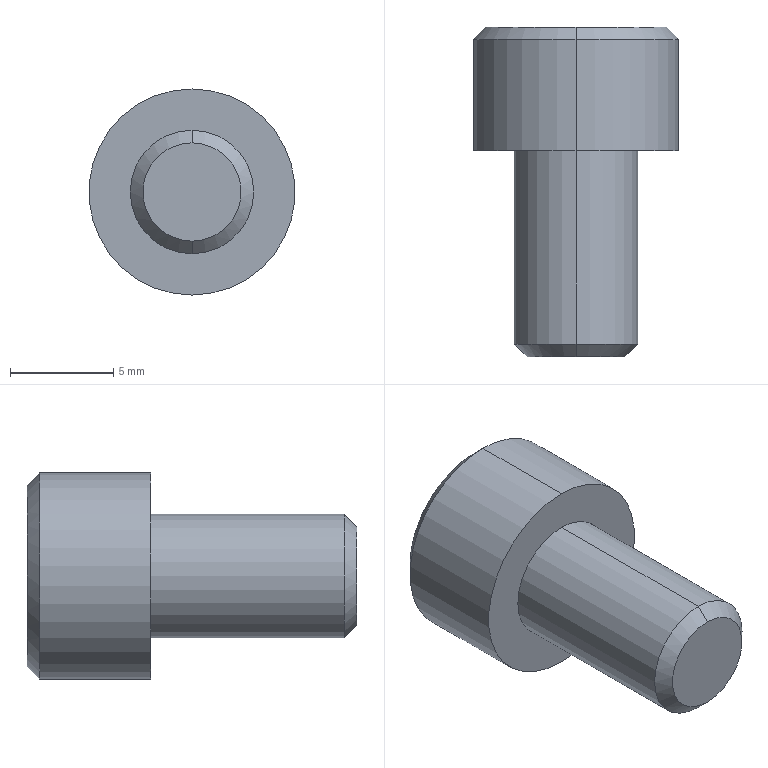Part | STEP file | PN59104-114_M_SHCSM6x1x10 | 1 solid | 18 faces | box 10 x 16 x 10 mm | volume 680.296 mm3 | plane 10 | cylinder 4 | cone 4 | commonest cylinder face diameters 6 x2 10 x2
STEP:
#1=CARTESIAN_POINT('',(0.,0.,-3.));
#2=VERTEX_POINT('',#1);
#3=CARTESIAN_POINT('',(0.,0.,3.));
#4=VERTEX_POINT('',#3);
#5=CARTESIAN_POINT('',(0.,0.,0.));
#6=DIRECTION('',(0.,-1.,0.));
#7=DIRECTION('',(0.,0.,-1.));
#8=AXIS2_PLACEMENT_3D('',#5,#6,#7);
#9=CIRCLE('',#8,3.);
#10=EDGE_CURVE('',#2,#4,#9,.T.);
#11=ORIENTED_EDGE('',*,*,#10,.T.);
#12=CARTESIAN_POINT('',(0.,-9.387,3.));
#13=VERTEX_POINT('',#12);
#14=CARTESIAN_POINT('',(0.,-10.,3.));
#15=DIRECTION('',(0.,-1.,0.));
#16=VECTOR('',#15,1000.);
#17=LINE('',#14,#16);
#18=EDGE_CURVE('',#4,#13,#17,.T.);
#19=ORIENTED_EDGE('',*,*,#18,.T.);
#20=CARTESIAN_POINT('',(0.,-9.387,-3.));
#21=VERTEX_POINT('',#20);
#22=CARTESIAN_POINT('',(0.,-9.387,0.));
#23=DIRECTION('',(0.,1.,0.));
#24=DIRECTION('',(0.,0.,-1.));
#25=AXIS2_PLACEMENT_3D('',#22,#23,#24);
#26=CIRCLE('',#25,3.);
#27=EDGE_CURVE('',#13,#21,#26,.T.);
#28=ORIENTED_EDGE('',*,*,#27,.T.);
#29=CARTESIAN_POINT('',(0.,-10.,-3.));
#30=DIRECTION('',(0.,-1.,0.));
#31=VECTOR('',#30,1000.);
#32=LINE('',#29,#31);
#33=EDGE_CURVE('',#2,#21,#32,.T.);
#34=ORIENTED_EDGE('',*,*,#33,.F.);
#35=EDGE_LOOP('',(#11,#19,#28,#34));
#36=FACE_OUTER_BOUND('',#35,.T.);
#37=CARTESIAN_POINT('',(0.,-10.,0.));
#38=DIRECTION('',(0.,-1.,0.));
#39=DIRECTION('',(0.,0.,-1.));
#40=AXIS2_PLACEMENT_3D('',#37,#38,#39);
#41=CYLINDRICAL_SURFACE('',#40,3.);
#42=ADVANCED_FACE('',(#36),#41,.T.);
#43=CARTESIAN_POINT('',(0.,-10.,2.387));
#44=VERTEX_POINT('',#43);
#45=CARTESIAN_POINT('',(0.,-10.,-2.387));
#46=VERTEX_POINT('',#45);
#47=CARTESIAN_POINT('',(0.,-10.,0.));
#48=DIRECTION('',(0.,1.,0.));
#49=DIRECTION('',(0.,0.,1.));
#50=AXIS2_PLACEMENT_3D('',#47,#48,#49);
#51=CIRCLE('',#50,2.387);
#52=EDGE_CURVE('',#44,#46,#51,.T.);
#53=ORIENTED_EDGE('',*,*,#52,.T.);
#54=CARTESIAN_POINT('',(0.,-9.387,-3.));
#55=DIRECTION('',(0.,0.7071,-0.7071));
#56=VECTOR('',#55,1000.);
#57=LINE('',#54,#56);
#58=EDGE_CURVE('',#46,#21,#57,.T.);
#59=ORIENTED_EDGE('',*,*,#58,.T.);
#60=ORIENTED_EDGE('',*,*,#27,.F.);
#61=CARTESIAN_POINT('',(0.,-9.387,3.));
#62=DIRECTION('',(0.,0.7071,0.7071));
#63=VECTOR('',#62,1000.);
#64=LINE('',#61,#63);
#65=EDGE_CURVE('',#44,#13,#64,.T.);
#66=ORIENTED_EDGE('',*,*,#65,.F.);
#67=EDGE_LOOP('',(#53,#59,#60,#66));
#68=FACE_OUTER_BOUND('',#67,.T.);
#69=CARTESIAN_POINT('',(0.,-9.387,0.));
#70=DIRECTION('',(0.,1.,0.));
#71=DIRECTION('',(0.,0.,1.));
#72=AXIS2_PLACEMENT_3D('',#69,#70,#71);
#73=CONICAL_SURFACE('',#72,3.,0.7854);
#74=ADVANCED_FACE('',(#68),#73,.T.);
#75=CARTESIAN_POINT('',(0.,5.4,-5.));
#76=VERTEX_POINT('',#75);
#77=CARTESIAN_POINT('',(0.,5.4,5.));
#78=VERTEX_POINT('',#77);
#79=CARTESIAN_POINT('',(0.,5.4,0.));
#80=DIRECTION('',(0.,-1.,0.));
#81=DIRECTION('',(0.,0.,-1.));
#82=AXIS2_PLACEMENT_3D('',#79,#80,#81);
#83=CIRCLE('',#82,5.);
#84=EDGE_CURVE('',#76,#78,#83,.T.);
#85=ORIENTED_EDGE('',*,*,#84,.T.);
#86=CARTESIAN_POINT('',(0.,0.,5.));
#87=VERTEX_POINT('',#86);
#88=CARTESIAN_POINT('',(0.,-10.,5.));
#89=DIRECTION('',(0.,-1.,0.));
#90=VECTOR('',#89,1000.);
#91=LINE('',#88,#90);
#92=EDGE_CURVE('',#78,#87,#91,.T.);
#93=ORIENTED_EDGE('',*,*,#92,.T.);
#94=CARTESIAN_POINT('',(0.,0.,-5.));
#95=VERTEX_POINT('',#94);
#96=CARTESIAN_POINT('',(0.,0.,0.));
#97=DIRECTION('',(0.,1.,0.));
#98=DIRECTION('',(0.,0.,-1.));
#99=AXIS2_PLACEMENT_3D('',#96,#97,#98);
#100=CIRCLE('',#99,5.);
#101=EDGE_CURVE('',#87,#95,#100,.T.);
#102=ORIENTED_EDGE('',*,*,#101,.T.);
#103=CARTESIAN_POINT('',(0.,-10.,-5.));
#104=DIRECTION('',(0.,-1.,0.));
#105=VECTOR('',#104,1000.);
#106=LINE('',#103,#105);
#107=EDGE_CURVE('',#76,#95,#106,.T.);
#108=ORIENTED_EDGE('',*,*,#107,.F.);
#109=EDGE_LOOP('',(#85,#93,#102,#108));
#110=FACE_OUTER_BOUND('',#109,.T.);
#111=CARTESIAN_POINT('',(0.,-10.,0.));
#112=DIRECTION('',(0.,-1.,0.));
#113=DIRECTION('',(0.,0.,-1.));
#114=AXIS2_PLACEMENT_3D('',#111,#112,#113);
#115=CYLINDRICAL_SURFACE('',#114,5.);
#116=ADVANCED_FACE('',(#110),#115,.T.);
#117=CARTESIAN_POINT('',(0.,6.,-4.4));
#118=VERTEX_POINT('',#117);
#119=CARTESIAN_POINT('',(0.,6.,4.4));
#120=VERTEX_POINT('',#119);
#121=CARTESIAN_POINT('',(0.,6.,0.));
#122=DIRECTION('',(0.,-1.,0.));
#123=DIRECTION('',(0.,0.,-1.));
#124=AXIS2_PLACEMENT_3D('',#121,#122,#123);
#125=CIRCLE('',#124,4.4);
#126=EDGE_CURVE('',#118,#120,#125,.T.);
#127=ORIENTED_EDGE('',*,*,#126,.T.);
#128=CARTESIAN_POINT('',(0.,5.4,5.));
#129=DIRECTION('',(0.,-0.7071,0.7071));
#130=VECTOR('',#129,1000.);
#131=LINE('',#128,#130);
#132=EDGE_CURVE('',#120,#78,#131,.T.);
#133=ORIENTED_EDGE('',*,*,#132,.T.);
#134=ORIENTED_EDGE('',*,*,#84,.F.);
#135=CARTESIAN_POINT('',(0.,5.4,-5.));
#136=DIRECTION('',(0.,-0.7071,-0.7071));
#137=VECTOR('',#136,1000.);
#138=LINE('',#135,#137);
#139=EDGE_CURVE('',#118,#76,#138,.T.);
#140=ORIENTED_EDGE('',*,*,#139,.F.);
#141=EDGE_LOOP('',(#127,#133,#134,#140));
#142=FACE_OUTER_BOUND('',#141,.T.);
#143=CARTESIAN_POINT('',(0.,5.4,0.));
#144=DIRECTION('',(0.,-1.,0.));
#145=DIRECTION('',(0.,0.,-1.));
#146=AXIS2_PLACEMENT_3D('',#143,#144,#145);
#147=CONICAL_SURFACE('',#146,5.,0.7854);
#148=ADVANCED_FACE('',(#142),#147,.T.);
#149=ORIENTED_EDGE('',*,*,#18,.F.);
#150=CARTESIAN_POINT('',(0.,0.,0.));
#151=DIRECTION('',(0.,-1.,0.));
#152=DIRECTION('',(0.,0.,-1.));
#153=AXIS2_PLACEMENT_3D('',#150,#151,#152);
#154=CIRCLE('',#153,3.);
#155=EDGE_CURVE('',#4,#2,#154,.T.);
#156=ORIENTED_EDGE('',*,*,#155,.T.);
#157=ORIENTED_EDGE('',*,*,#33,.T.);
#158=CARTESIAN_POINT('',(0.,-9.387,0.));
#159=DIRECTION('',(0.,1.,0.));
#160=DIRECTION('',(0.,0.,-1.));
#161=AXIS2_PLACEMENT_3D('',#158,#159,#160);
#162=CIRCLE('',#161,3.);
#163=EDGE_CURVE('',#21,#13,#162,.T.);
#164=ORIENTED_EDGE('',*,*,#163,.T.);
#165=EDGE_LOOP('',(#149,#156,#157,#164));
#166=FACE_OUTER_BOUND('',#165,.T.);
#167=CARTESIAN_POINT('',(0.,-10.,0.));
#168=DIRECTION('',(0.,-1.,0.));
#169=DIRECTION('',(0.,0.,-1.));
#170=AXIS2_PLACEMENT_3D('',#167,#168,#169);
#171=CYLINDRICAL_SURFACE('',#170,3.);
#172=ADVANCED_FACE('',(#166),#171,.T.);
#173=CARTESIAN_POINT('',(0.,0.,0.));
#174=DIRECTION('',(0.,1.,0.));
#175=DIRECTION('',(0.,0.,-1.));
#176=AXIS2_PLACEMENT_3D('',#173,#174,#175);
#177=CIRCLE('',#176,5.);
#178=EDGE_CURVE('',#95,#87,#177,.T.);
#179=ORIENTED_EDGE('',*,*,#178,.F.);
#180=ORIENTED_EDGE('',*,*,#101,.F.);
#181=EDGE_LOOP('',(#179,#180));
#182=FACE_OUTER_BOUND('',#181,.T.);
#183=ORIENTED_EDGE('',*,*,#10,.F.);
#184=ORIENTED_EDGE('',*,*,#155,.F.);
#185=EDGE_LOOP('',(#183,#184));
#186=FACE_BOUND('',#185,.T.);
#187=CARTESIAN_POINT('',(5.,0.,0.));
#188=DIRECTION('',(0.,1.,0.));
#189=DIRECTION('',(0.,0.,1.));
#190=AXIS2_PLACEMENT_3D('',#187,#188,#189);
#191=PLANE('',#190);
#192=ADVANCED_FACE('',(#182,#186),#191,.F.);
#193=ORIENTED_EDGE('',*,*,#58,.F.);
#194=CARTESIAN_POINT('',(0.,-10.,0.));
#195=DIRECTION('',(0.,1.,0.));
#196=DIRECTION('',(0.,0.,1.));
#197=AXIS2_PLACEMENT_3D('',#194,#195,#196);
#198=CIRCLE('',#197,2.387);
#199=EDGE_CURVE('',#46,#44,#198,.T.);
#200=ORIENTED_EDGE('',*,*,#199,.T.);
#201=ORIENTED_EDGE('',*,*,#65,.T.);
#202=ORIENTED_EDGE('',*,*,#163,.F.);
#203=EDGE_LOOP('',(#193,#200,#201,#202));
#204=FACE_OUTER_BOUND('',#203,.T.);
#205=CARTESIAN_POINT('',(0.,-9.387,0.));
#206=DIRECTION('',(0.,1.,0.));
#207=DIRECTION('',(0.,0.,1.));
#208=AXIS2_PLACEMENT_3D('',#205,#206,#207);
#209=CONICAL_SURFACE('',#208,3.,0.7854);
#210=ADVANCED_FACE('',(#204),#209,.T.);
#211=ORIENTED_EDGE('',*,*,#92,.F.);
#212=CARTESIAN_POINT('',(0.,5.4,0.));
#213=DIRECTION('',(0.,-1.,0.));
#214=DIRECTION('',(0.,0.,-1.));
#215=AXIS2_PLACEMENT_3D('',#212,#213,#214);
#216=CIRCLE('',#215,5.);
#217=EDGE_CURVE('',#78,#76,#216,.T.);
#218=ORIENTED_EDGE('',*,*,#217,.T.);
#219=ORIENTED_EDGE('',*,*,#107,.T.);
#220=ORIENTED_EDGE('',*,*,#178,.T.);
#221=EDGE_LOOP('',(#211,#218,#219,#220));
#222=FACE_OUTER_BOUND('',#221,.T.);
#223=CARTESIAN_POINT('',(0.,-10.,0.));
#224=DIRECTION('',(0.,-1.,0.));
#225=DIRECTION('',(0.,0.,-1.));
#226=AXIS2_PLACEMENT_3D('',#223,#224,#225);
#227=CYLINDRICAL_SURFACE('',#226,5.);
#228=ADVANCED_FACE('',(#222),#227,.T.);
#229=ORIENTED_EDGE('',*,*,#52,.F.);
#230=ORIENTED_EDGE('',*,*,#199,.F.);
#231=EDGE_LOOP('',(#229,#230));
#232=FACE_OUTER_BOUND('',#231,.T.);
#233=CARTESIAN_POINT('',(2.386,-10.,0.));
#234=DIRECTION('',(0.,1.,0.));
#235=DIRECTION('',(0.,0.,1.));
#236=AXIS2_PLACEMENT_3D('',#233,#234,#235);
#237=PLANE('',#236);
#238=ADVANCED_FACE('',(#232),#237,.F.);
#239=ORIENTED_EDGE('',*,*,#132,.F.);
#240=CARTESIAN_POINT('',(0.,6.,0.));
#241=DIRECTION('',(0.,-1.,0.));
#242=DIRECTION('',(0.,0.,-1.));
#243=AXIS2_PLACEMENT_3D('',#240,#241,#242);
#244=CIRCLE('',#243,4.4);
#245=EDGE_CURVE('',#120,#118,#244,.T.);
#246=ORIENTED_EDGE('',*,*,#245,.T.);
#247=ORIENTED_EDGE('',*,*,#139,.T.);
#248=ORIENTED_EDGE('',*,*,#217,.F.);
#249=EDGE_LOOP('',(#239,#246,#247,#248));
#250=FACE_OUTER_BOUND('',#249,.T.);
#251=CARTESIAN_POINT('',(0.,5.4,0.));
#252=DIRECTION('',(0.,-1.,0.));
#253=DIRECTION('',(0.,0.,-1.));
#254=AXIS2_PLACEMENT_3D('',#251,#252,#253);
#255=CONICAL_SURFACE('',#254,5.,0.7854);
#256=ADVANCED_FACE('',(#250),#255,.T.);
#257=CARTESIAN_POINT('',(-2.5,6.,1.443));
#258=VERTEX_POINT('',#257);
#259=CARTESIAN_POINT('',(0.,6.,2.887));
#260=VERTEX_POINT('',#259);
#261=CARTESIAN_POINT('',(-2.5,6.,1.443));
#262=DIRECTION('',(0.866,0.,0.5));
#263=VECTOR('',#262,1000.);
#264=LINE('',#261,#263);
#265=EDGE_CURVE('',#258,#260,#264,.T.);
#266=ORIENTED_EDGE('',*,*,#265,.F.);
#267=CARTESIAN_POINT('',(-2.5,6.,-1.443));
#268=VERTEX_POINT('',#267);
#269=CARTESIAN_POINT('',(-2.5,6.,0.));
#270=DIRECTION('',(0.,0.,1.));
#271=VECTOR('',#270,1000.);
#272=LINE('',#269,#271);
#273=EDGE_CURVE('',#268,#258,#272,.T.);
#274=ORIENTED_EDGE('',*,*,#273,.F.);
#275=CARTESIAN_POINT('',(0.,6.,-2.887));
#276=VERTEX_POINT('',#275);
#277=CARTESIAN_POINT('',(0.,6.,-2.887));
#278=DIRECTION('',(-0.866,0.,0.5));
#279=VECTOR('',#278,1000.);
#280=LINE('',#277,#279);
#281=EDGE_CURVE('',#276,#268,#280,.T.);
#282=ORIENTED_EDGE('',*,*,#281,.F.);
#283=CARTESIAN_POINT('',(2.5,6.,-1.443));
#284=VERTEX_POINT('',#283);
#285=CARTESIAN_POINT('',(2.5,6.,-1.443));
#286=DIRECTION('',(-0.866,0.,-0.5));
#287=VECTOR('',#286,1000.);
#288=LINE('',#285,#287);
#289=EDGE_CURVE('',#284,#276,#288,.T.);
#290=ORIENTED_EDGE('',*,*,#289,.F.);
#291=CARTESIAN_POINT('',(2.5,6.,1.443));
#292=VERTEX_POINT('',#291);
#293=CARTESIAN_POINT('',(2.5,6.,0.));
#294=DIRECTION('',(0.,0.,-1.));
#295=VECTOR('',#294,1000.);
#296=LINE('',#293,#295);
#297=EDGE_CURVE('',#292,#284,#296,.T.);
#298=ORIENTED_EDGE('',*,*,#297,.F.);
#299=CARTESIAN_POINT('',(0.,6.,2.887));
#300=DIRECTION('',(0.866,0.,-0.5));
#301=VECTOR('',#300,1000.);
#302=LINE('',#299,#301);
#303=EDGE_CURVE('',#260,#292,#302,.T.);
#304=ORIENTED_EDGE('',*,*,#303,.F.);
#305=EDGE_LOOP('',(#266,#274,#282,#290,#298,#304));
#306=FACE_BOUND('',#305,.T.);
#307=ORIENTED_EDGE('',*,*,#126,.F.);
#308=ORIENTED_EDGE('',*,*,#245,.F.);
#309=EDGE_LOOP('',(#307,#308));
#310=FACE_OUTER_BOUND('',#309,.T.);
#311=CARTESIAN_POINT('',(0.,6.,0.));
#312=DIRECTION('',(0.,-1.,0.));
#313=DIRECTION('',(0.,0.,-1.));
#314=AXIS2_PLACEMENT_3D('',#311,#312,#313);
#315=PLANE('',#314);
#316=ADVANCED_FACE('',(#306,#310),#315,.F.);
#317=CARTESIAN_POINT('',(2.5,3.,1.443));
#318=VERTEX_POINT('',#317);
#319=CARTESIAN_POINT('',(2.5,3.,1.443));
#320=DIRECTION('',(0.,1.,0.));
#321=VECTOR('',#320,1000.);
#322=LINE('',#319,#321);
#323=EDGE_CURVE('',#318,#292,#322,.T.);
#324=ORIENTED_EDGE('',*,*,#323,.F.);
#325=CARTESIAN_POINT('',(0.,3.,2.887));
#326=VERTEX_POINT('',#325);
#327=CARTESIAN_POINT('',(0.,3.,2.887));
#328=DIRECTION('',(0.866,0.,-0.5));
#329=VECTOR('',#328,1000.);
#330=LINE('',#327,#329);
#331=EDGE_CURVE('',#326,#318,#330,.T.);
#332=ORIENTED_EDGE('',*,*,#331,.F.);
#333=CARTESIAN_POINT('',(0.,3.,2.887));
#334=DIRECTION('',(0.,-1.,0.));
#335=VECTOR('',#334,1000.);
#336=LINE('',#333,#335);
#337=EDGE_CURVE('',#260,#326,#336,.T.);
#338=ORIENTED_EDGE('',*,*,#337,.F.);
#339=ORIENTED_EDGE('',*,*,#303,.T.);
#340=EDGE_LOOP('',(#324,#332,#338,#339));
#341=FACE_OUTER_BOUND('',#340,.T.);
#342=CARTESIAN_POINT('',(0.,3.,2.887));
#343=DIRECTION('',(0.5,0.,0.866));
#344=DIRECTION('',(0.866,0.,-0.5));
#345=AXIS2_PLACEMENT_3D('',#342,#343,#344);
#346=PLANE('',#345);
#347=ADVANCED_FACE('',(#341),#346,.F.);
#348=ORIENTED_EDGE('',*,*,#337,.T.);
#349=CARTESIAN_POINT('',(-2.5,3.,1.443));
#350=VERTEX_POINT('',#349);
#351=CARTESIAN_POINT('',(-2.5,3.,1.443));
#352=DIRECTION('',(0.866,0.,0.5));
#353=VECTOR('',#352,1000.);
#354=LINE('',#351,#353);
#355=EDGE_CURVE('',#350,#326,#354,.T.);
#356=ORIENTED_EDGE('',*,*,#355,.F.);
#357=CARTESIAN_POINT('',(-2.5,3.,1.443));
#358=DIRECTION('',(0.,-1.,0.));
#359=VECTOR('',#358,1000.);
#360=LINE('',#357,#359);
#361=EDGE_CURVE('',#258,#350,#360,.T.);
#362=ORIENTED_EDGE('',*,*,#361,.F.);
#363=ORIENTED_EDGE('',*,*,#265,.T.);
#364=EDGE_LOOP('',(#348,#356,#362,#363));
#365=FACE_OUTER_BOUND('',#364,.T.);
#366=CARTESIAN_POINT('',(-2.5,3.,1.443));
#367=DIRECTION('',(-0.5,0.,0.866));
#368=DIRECTION('',(0.866,0.,0.5));
#369=AXIS2_PLACEMENT_3D('',#366,#367,#368);
#370=PLANE('',#369);
#371=ADVANCED_FACE('',(#365),#370,.F.);
#372=ORIENTED_EDGE('',*,*,#361,.T.);
#373=CARTESIAN_POINT('',(-2.5,3.,-1.443));
#374=VERTEX_POINT('',#373);
#375=CARTESIAN_POINT('',(-2.5,3.,-1.443));
#376=DIRECTION('',(0.,0.,1.));
#377=VECTOR('',#376,1000.);
#378=LINE('',#375,#377);
#379=EDGE_CURVE('',#374,#350,#378,.T.);
#380=ORIENTED_EDGE('',*,*,#379,.F.);
#381=CARTESIAN_POINT('',(-2.5,3.,-1.443));
#382=DIRECTION('',(0.,-1.,0.));
#383=VECTOR('',#382,1000.);
#384=LINE('',#381,#383);
#385=EDGE_CURVE('',#268,#374,#384,.T.);
#386=ORIENTED_EDGE('',*,*,#385,.F.);
#387=ORIENTED_EDGE('',*,*,#273,.T.);
#388=EDGE_LOOP('',(#372,#380,#386,#387));
#389=FACE_OUTER_BOUND('',#388,.T.);
#390=CARTESIAN_POINT('',(-2.5,3.,-1.443));
#391=DIRECTION('',(-1.,0.,0.));
#392=DIRECTION('',(0.,0.,1.));
#393=AXIS2_PLACEMENT_3D('',#390,#391,#392);
#394=PLANE('',#393);
#395=ADVANCED_FACE('',(#389),#394,.F.);
#396=ORIENTED_EDGE('',*,*,#385,.T.);
#397=CARTESIAN_POINT('',(0.,3.,-2.887));
#398=VERTEX_POINT('',#397);
#399=CARTESIAN_POINT('',(0.,3.,-2.887));
#400=DIRECTION('',(-0.866,0.,0.5));
#401=VECTOR('',#400,1000.);
#402=LINE('',#399,#401);
#403=EDGE_CURVE('',#398,#374,#402,.T.);
#404=ORIENTED_EDGE('',*,*,#403,.F.);
#405=CARTESIAN_POINT('',(0.,3.,-2.887));
#406=DIRECTION('',(0.,-1.,0.));
#407=VECTOR('',#406,1000.);
#408=LINE('',#405,#407);
#409=EDGE_CURVE('',#276,#398,#408,.T.);
#410=ORIENTED_EDGE('',*,*,#409,.F.);
#411=ORIENTED_EDGE('',*,*,#281,.T.);
#412=EDGE_LOOP('',(#396,#404,#410,#411));
#413=FACE_OUTER_BOUND('',#412,.T.);
#414=CARTESIAN_POINT('',(0.,3.,-2.887));
#415=DIRECTION('',(-0.5,0.,-0.866));
#416=DIRECTION('',(-0.866,0.,0.5));
#417=AXIS2_PLACEMENT_3D('',#414,#415,#416);
#418=PLANE('',#417);
#419=ADVANCED_FACE('',(#413),#418,.F.);
#420=ORIENTED_EDGE('',*,*,#409,.T.);
#421=CARTESIAN_POINT('',(2.5,3.,-1.443));
#422=VERTEX_POINT('',#421);
#423=CARTESIAN_POINT('',(2.5,3.,-1.443));
#424=DIRECTION('',(-0.866,0.,-0.5));
#425=VECTOR('',#424,1000.);
#426=LINE('',#423,#425);
#427=EDGE_CURVE('',#422,#398,#426,.T.);
#428=ORIENTED_EDGE('',*,*,#427,.F.);
#429=CARTESIAN_POINT('',(2.5,3.,-1.443));
#430=DIRECTION('',(0.,-1.,0.));
#431=VECTOR('',#430,1000.);
#432=LINE('',#429,#431);
#433=EDGE_CURVE('',#284,#422,#432,.T.);
#434=ORIENTED_EDGE('',*,*,#433,.F.);
#435=ORIENTED_EDGE('',*,*,#289,.T.);
#436=EDGE_LOOP('',(#420,#428,#434,#435));
#437=FACE_OUTER_BOUND('',#436,.T.);
#438=CARTESIAN_POINT('',(2.5,3.,-1.443));
#439=DIRECTION('',(0.5,0.,-0.866));
#440=DIRECTION('',(-0.866,0.,-0.5));
#441=AXIS2_PLACEMENT_3D('',#438,#439,#440);
#442=PLANE('',#441);
#443=ADVANCED_FACE('',(#437),#442,.F.);
#444=ORIENTED_EDGE('',*,*,#297,.T.);
#445=ORIENTED_EDGE('',*,*,#433,.T.);
#446=CARTESIAN_POINT('',(2.5,3.,1.443));
#447=DIRECTION('',(0.,0.,-1.));
#448=VECTOR('',#447,1000.);
#449=LINE('',#446,#448);
#450=EDGE_CURVE('',#318,#422,#449,.T.);
#451=ORIENTED_EDGE('',*,*,#450,.F.);
#452=ORIENTED_EDGE('',*,*,#323,.T.);
#453=EDGE_LOOP('',(#444,#445,#451,#452));
#454=FACE_OUTER_BOUND('',#453,.T.);
#455=CARTESIAN_POINT('',(2.5,3.,1.443));
#456=DIRECTION('',(1.,0.,0.));
#457=DIRECTION('',(0.,0.,-1.));
#458=AXIS2_PLACEMENT_3D('',#455,#456,#457);
#459=PLANE('',#458);
#460=ADVANCED_FACE('',(#454),#459,.F.);
#461=ORIENTED_EDGE('',*,*,#427,.T.);
#462=ORIENTED_EDGE('',*,*,#403,.T.);
#463=ORIENTED_EDGE('',*,*,#379,.T.);
#464=ORIENTED_EDGE('',*,*,#355,.T.);
#465=ORIENTED_EDGE('',*,*,#331,.T.);
#466=ORIENTED_EDGE('',*,*,#450,.T.);
#467=EDGE_LOOP('',(#461,#462,#463,#464,#465,#466));
#468=FACE_OUTER_BOUND('',#467,.T.);
#469=CARTESIAN_POINT('',(0.,3.,0.));
#470=DIRECTION('',(0.,1.,0.));
#471=DIRECTION('',(0.,0.,1.));
#472=AXIS2_PLACEMENT_3D('',#469,#470,#471);
#473=PLANE('',#472);
#474=ADVANCED_FACE('',(#468),#473,.T.);
#475=CLOSED_SHELL('',(#42,#74,#116,#148,#172,#192,#210,#228,#238,#256,#316,#347,#371,#395,#419,#443,#460,#474));
#476=MANIFOLD_SOLID_BREP('',#475);
#477=CARTESIAN_POINT('',(0.,0.,0.));
#478=DIRECTION('',(0.,0.,1.));
#479=DIRECTION('',(1.,0.,0.));
#480=AXIS2_PLACEMENT_3D('',#477,#478,#479);
#481=(LENGTH_UNIT()NAMED_UNIT(*)SI_UNIT(.MILLI.,.METRE.));
#482=UNCERTAINTY_MEASURE_WITH_UNIT(LENGTH_MEASURE(0.00001),#481,'','');
#483=(NAMED_UNIT(*)PLANE_ANGLE_UNIT()SI_UNIT($,.RADIAN.));
#484=(NAMED_UNIT(*)SI_UNIT($,.STERADIAN.)SOLID_ANGLE_UNIT());
#485=(GEOMETRIC_REPRESENTATION_CONTEXT(3)GLOBAL_UNCERTAINTY_ASSIGNED_CONTEXT((#482))GLOBAL_UNIT_ASSIGNED_CONTEXT((#481,#483,#484))REPRESENTATION_CONTEXT('',''));
#486=ADVANCED_BREP_SHAPE_REPRESENTATION('',(#476,#480),#485);